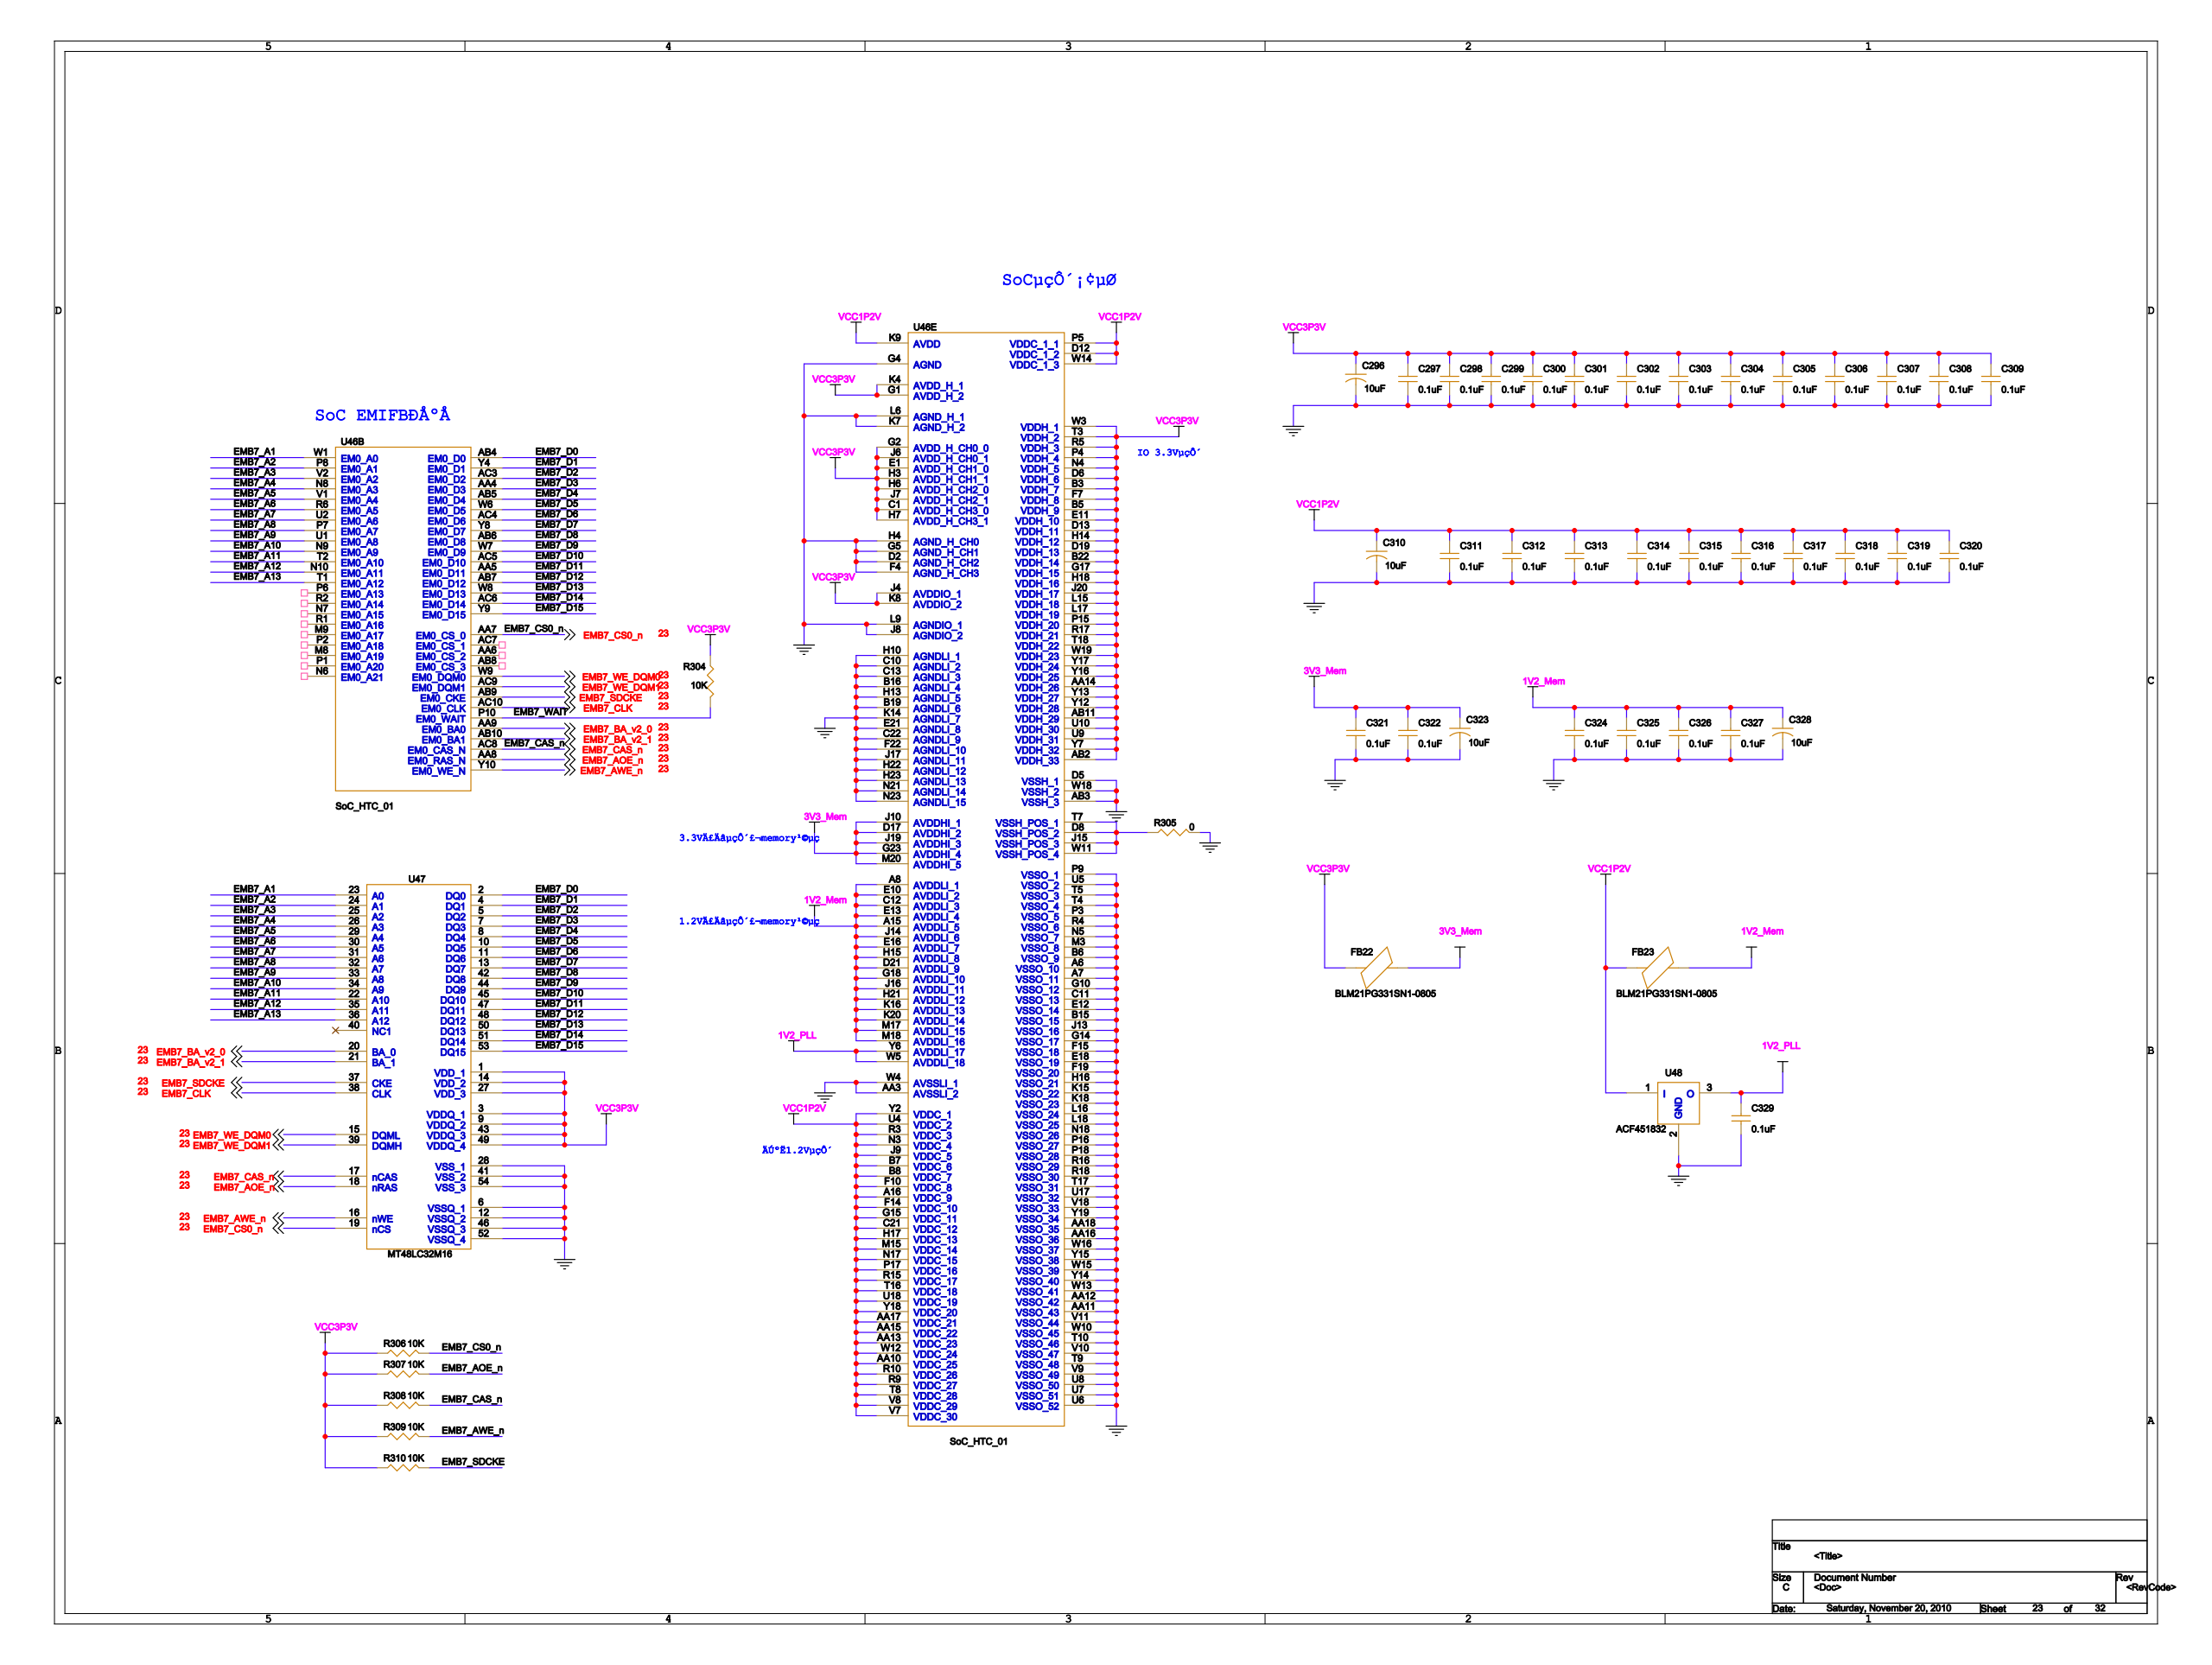Circuit board | Cadence Allegro | 1001 parts | 1318 nets | one sheet of the schematic
Parts on this sheet (reference | value | footprint):
C1 | 10uF | C3216
C10 | 0.1uF | C0402
C21 | 0.1uF | C0402
C22 | 0.1uF | C0402
C296 | 10uF | C3216
C297 | 0.1uF | C0402
C298 | 0.1uF | C0402
C299 | 0.1uF | C0402
C300 | 0.1uF | C0402
C301 | 0.1uF | C0402
C302 | 0.1uF | C0402
C303 | 0.1uF | C0402
C304 | 0.1uF | C0402
C305 | 0.1uF | C0402
C306 | 0.1uF | C0402
C307 | 0.1uF | C0402
C308 | 0.1uF | C0402
C309 | 0.1uF | C0402
C310 | 10uF | C3216
C311 | 0.1uF | C0402
C312 | 0.1uF | C0402
C313 | 0.1uF | C0402
C314 | 0.1uF | C0402
C315 | 0.1uF | C0402
C316 | 0.1uF | C0402
C317 | 0.1uF | C0402
C318 | 0.1uF | C0402
C319 | 0.1uF | C0402
C320 | 0.1uF | C0402
C321 | 0.1uF | C0402
C322 | 0.1uF | C0402
C323 | 10uF | C3216
C324 | 0.1uF | C0402
C325 | 0.1uF | C0402
C326 | 0.1uF | C0402
C327 | 0.1uF | C0402
C328 | 10uF | C3216
C329 | 0.1uF | 0603
FB22 | BLM21PG331SN1-0805 | 1210
FB23 | BLM21PG331SN1-0805 | 1210
R304 | 10K | 0603
R305 | 0 | 0603
R306 | 10K | 0603
R307 | 10K | 0603
R308 | 10K | 0603
R309 | 10K | 0603
R310 | 10K | 0603
U1 | SoC_HTC_01 | L529_XIN
U2 | MT48LC32M16 | TSOP54
U4 | MAX3243 | TSSOP-28
U6 | MT48LC16M16 | TSOP54
U7 | MT48LC16M16 | TSOP54
U8 | DP83848C | DP83848C_48LQFP
U10 | SoC_HTC_01 | L529_XIN
U17 | MT48LC32M16 | TSOP54
U46 | SoC_HTC_01 | L529_XIN
U47 | MT48LC32M16 | TSOP54
U48 | ACF451832 | EMI_FILTER
Nets of these parts (net: part-pin ...):
GND: C1-2 C10-2 C21-2 C22-2 C296-2 C297-2 C298-2 C299-2 C300-2 C301-2 C302-2 C303-2 C304-2 C305-2 C306-2 C307-2 C308-2 C309-2 C310-2 C311-2 C312-2 C313-2 C314-2 C315-2 C316-2 C317-2 C318-2 C319-2 C320-2 C321-2 C322-2 C323-2 C324-2 C325-2 C326-2 C327-2 C328-2 C329-2 R305-2 U48-2 U1-A6 U1-A7 U1-AA3 U1-AA11 U1-AA12 U1-AA16 U1-AA18 U1-AB3 U1-B6 U1-B15 U1-B16 U1-B19 U1-C10 U1-C11 U1-C13 U1-C22 U1-D2 U1-D5 U1-E12 U1-E18 U1-E21 U1-F4 U1-F15 U1-F19 U1-F22 U1-G4 U1-G5 U1-G10 U1-G14 U1-H4 U1-H10 U1-H13 U1-H16 U1-H22 U1-H23 U1-J8 U1-J13 U1-J17 U1-K7 U1-K14 U1-K15 U1-K18 U1-L6 U1-L9 U1-L16 U1-L18 U1-M3 U1-N5 U1-N18 U1-N21 U1-N23 U1-P3 U1-P9 U1-P16 U1-P18 U1-R4 U1-R16 U1-R18 U1-T4 U1-T5 U1-T9 U1-T10 U1-T17 U1-U5 U1-U6 U1-U7 U1-U8 U1-U17 U1-V9 U1-V10 U1-V11 U1-V18 U1-W4 U1-W10 U1-W13 U1-W15 U1-W16 U1-W18 U1-Y14 U1-Y15 U1-Y19 U2-6 U2-12 U2-28 U2-41 U2-46 U2-52 U2-54 U4-23 U4-25 U6-6 U6-12 U6-28 U6-41 U6-46 U6-52 U6-54 U7-6 U7-12 U7-28 U7-41 U7-46 U7-52 U7-54 U8-15 U8-19 U8-35 U8-36 U8-47 U10-A6 U10-A7 U10-AA3 U10-AA11 U10-AA12 U10-AA16 U10-AA18 U10-AB3 U10-B6 U10-B15 U10-B16 U10-B19 U10-C10 U10-C11 U10-C13 U10-C22 U10-D2 U10-D5 U10-E12 U10-E18 U10-E21 U10-F4 U10-F15 U10-F19 U10-F22 U10-G4 U10-G5 U10-G10 U10-G14 U10-H4 U10-H10 U10-H13 U10-H16 U10-H22 U10-H23 U10-J8 U10-J13 U10-J17 U10-K7 U10-K14 U10-K15 U10-K18 U10-L6 U10-L9 U10-L16 U10-L18 U10-M3 U10-N5 U10-N18 U10-N21 U10-N23 U10-P3 U10-P9 U10-P16 U10-P18 U10-R4 U10-R16 U10-R18 U10-T4 U10-T5 U10-T9 U10-T10 U10-T17 U10-U5 U10-U6 U10-U7 U10-U8 U10-U17 U10-V9 U10-V10 U10-V11 U10-V18 U10-W4 U10-W10 U10-W13 U10-W15 U10-W16 U10-W18 U10-Y14 U10-Y15 U10-Y19 U17-6 U17-12 U17-28 U17-41 U17-46 U17-52 U17-54 U46-A6 U46-A7 U46-AA3 U46-AA11 U46-AA12 U46-AA16 U46-AA18 U46-AB3 U46-B6 U46-B15 U46-B16 U46-B19 U46-C10 U46-C11 U46-C13 U46-C22 U46-D2 U46-D5 U46-E12 U46-E18 U46-E21 U46-F4 U46-F15 U46-F19 U46-F22 U46-G4 U46-G5 U46-G10 U46-G14 U46-H4 U46-H10 U46-H13 U46-H16 U46-H22 U46-H23 U46-J8 U46-J13 U46-J17 U46-K7 U46-K14 U46-K15 U46-K18 U46-L6 U46-L9 U46-L16 U46-L18 U46-M3 U46-N5 U46-N18 U46-N21 U46-N23 U46-P3 U46-P9 U46-P16 U46-P18 U46-R4 U46-R16 U46-R18 U46-T4 U46-T5 U46-T9 U46-T10 U46-T17 U46-U5 U46-U6 U46-U7 U46-U8 U46-U17 U46-V9 U46-V10 U46-V11 U46-V18 U46-W4 U46-W10 U46-W13 U46-W15 U46-W16 U46-W18 U46-Y14 U46-Y15 U46-Y19 U47-6 U47-12 U47-28 U47-41 U47-46 U47-52 U47-54
VCC3P3V: C1-1 C10-1 C296-1 C297-1 C298-1 C299-1 C300-1 C301-1 C302-1 C303-1 C304-1 C305-1 C306-1 C307-1 C308-1 C309-1 FB22-1 R304-2 R306-1 R307-1 R308-1 R309-1 R310-1 U1-AA14 U1-AB2 U1-AB11 U1-B3 U1-B5 U1-B22 U1-C1 U1-D6 U1-D13 U1-D19 U1-E1 U1-E11 U1-F7 U1-G1 U1-G2 U1-G17 U1-H3 U1-H6 U1-H7 U1-H14 U1-H18 U1-J4 U1-J6 U1-J7 U1-J20 U1-K4 U1-K8 U1-L15 U1-L17 U1-N4 U1-P4 U1-P15 U1-R5 U1-R17 U1-T3 U1-T18 U1-U9 U1-U10 U1-W3 U1-W19 U1-Y7 U1-Y12 U1-Y13 U1-Y16 U1-Y17 U2-1 U2-3 U2-9 U2-14 U2-27 U2-43 U2-49 U4-22 U4-26 U6-1 U6-3 U6-9 U6-14 U6-27 U6-43 U6-49 U7-1 U7-3 U7-9 U7-14 U7-27 U7-43 U7-49 U8-22 U8-32 U8-48 U10-AA14 U10-AB2 U10-AB11 U10-B3 U10-B5 U10-B22 U10-C1 U10-D6 U10-D13 U10-D19 U10-E1 U10-E11 U10-F7 U10-G1 U10-G2 U10-G17 U10-H3 U10-H6 U10-H7 U10-H14 U10-H18 U10-J4 U10-J6 U10-J7 U10-J20 U10-K4 U10-K8 U10-L15 U10-L17 U10-N4 U10-P4 U10-P15 U10-R5 U10-R17 U10-T3 U10-T18 U10-U9 U10-U10 U10-W3 U10-W19 U10-Y7 U10-Y12 U10-Y13 U10-Y16 U10-Y17 U17-1 U17-3 U17-9 U17-14 U17-27 U17-43 U17-49 U46-AA14 U46-AB2 U46-AB11 U46-B3 U46-B5 U46-B22 U46-C1 U46-D6 U46-D13 U46-D19 U46-E1 U46-E11 U46-F7 U46-G1 U46-G2 U46-G17 U46-H3 U46-H6 U46-H7 U46-H14 U46-H18 U46-J4 U46-J6 U46-J7 U46-J20 U46-K4 U46-K8 U46-L15 U46-L17 U46-N4 U46-P4 U46-P15 U46-R5 U46-R17 U46-T3 U46-T18 U46-U9 U46-U10 U46-W3 U46-W19 U46-Y7 U46-Y12 U46-Y13 U46-Y16 U46-Y17 U47-1 U47-3 U47-9 U47-14 U47-27 U47-43 U47-49
VCC1P2V: C21-1 C22-1 C310-1 C311-1 C312-1 C313-1 C314-1 C315-1 C316-1 C317-1 C318-1 C319-1 C320-1 FB23-1 U48-1 U1-A16 U1-AA10 U1-AA13 U1-AA15 U1-AA17 U1-B7 U1-B8 U1-C21 U1-D12 U1-F10 U1-F14 U1-G15 U1-H17 U1-J9 U1-K9 U1-M15 U1-N3 U1-N17 U1-P5 U1-P17 U1-R3 U1-R9 U1-R10 U1-R15 U1-T8 U1-T16 U1-U4 U1-U18 U1-V7 U1-V8 U1-W12 U1-W14 U1-Y2 U1-Y18 U10-A16 U10-AA10 U10-AA13 U10-AA15 U10-AA17 U10-B7 U10-B8 U10-C21 U10-D12 U10-F10 U10-F14 U10-G15 U10-H17 U10-J9 U10-K9 U10-M15 U10-N3 U10-N17 U10-P5 U10-P17 U10-R3 U10-R9 U10-R10 U10-R15 U10-T8 U10-T16 U10-U4 U10-U18 U10-V7 U10-V8 U10-W12 U10-W14 U10-Y2 U10-Y18 U46-A16 U46-AA10 U46-AA13 U46-AA15 U46-AA17 U46-B7 U46-B8 U46-C21 U46-D12 U46-F10 U46-F14 U46-G15 U46-H17 U46-J9 U46-K9 U46-M15 U46-N3 U46-N17 U46-P5 U46-P17 U46-R3 U46-R9 U46-R10 U46-R15 U46-T8 U46-T16 U46-U4 U46-U18 U46-V7 U46-V8 U46-W12 U46-W14 U46-Y2 U46-Y18
3V3_MEM: C321-1 C322-1 C323-1 FB22-2 U1-D17 U1-G23 U1-J10 U1-J19 U1-M20 U10-D17 U10-G23 U10-J10 U10-J19 U10-M20 U46-D17 U46-G23 U46-J10 U46-J19 U46-M20
1V2_MEM: C324-1 C325-1 C326-1 C327-1 C328-1 FB23-2 U1-A8 U1-A15 U1-C12 U1-D21 U1-E10 U1-E13 U1-E16 U1-G18 U1-H15 U1-H21 U1-J14 U1-J16 U1-K16 U1-K20 U1-M17 U1-M18 U10-A8 U10-A15 U10-C12 U10-D21 U10-E10 U10-E13 U10-E16 U10-G18 U10-H15 U10-H21 U10-J14 U10-J16 U10-K16 U10-K20 U10-M17 U10-M18 U46-A8 U46-A15 U46-C12 U46-D21 U46-E10 U46-E13 U46-E16 U46-G18 U46-H15 U46-H21 U46-J14 U46-J16 U46-K16 U46-K20 U46-M17 U46-M18
1V2_PLL: C329-1 U48-3 U1-W5 U1-Y6 U10-W5 U10-Y6 U46-W5 U46-Y6
EMB7_A1: U46-W1 U47-23
EMB7_A2: U46-P8 U47-24
EMB7_A11: U46-T2 U47-22
EMB7_A12: U46-N10 U47-35
EMB7_A13: U46-T1 U47-36
EMB7_A3: U46-V2 U47-25
EMB7_A4: U46-N8 U47-26
EMB7_A5: U46-V1 U47-29
EMB7_A6: U46-R6 U47-30
EMB7_A7: U46-U2 U47-31
EMB7_A8: U46-P7 U47-32
EMB7_A9: U46-U1 U47-33
EMB7_A10: U46-N9 U47-34
EMB7_CAS_N: R308-2 U46-AC8 U47-17
EMB7_SDCKE: R310-2 U46-AB9 U47-37
EMB7_CLK: U46-AC10 U47-38
EMB7_CS0_N: R306-2 U46-AA7 U47-19
EMB7_D0: U46-AB4 U47-2
EMB7_D1: U46-Y4 U47-4
EMB7_D10: U46-AC5 U47-45
EMB7_D11: U46-AA5 U47-47
EMB7_D12: U46-AB7 U47-48
EMB7_D13: U46-W8 U47-50
EMB7_D14: U46-AC6 U47-51
EMB7_D15: U46-Y9 U47-53
EMB7_D2: U46-AC3 U47-5
EMB7_D3: U46-AA4 U47-7
EMB7_D4: U46-AB5 U47-8
EMB7_D5: U46-W6 U47-10
EMB7_D6: U46-AC4 U47-11
EMB7_D7: U46-Y8 U47-13
EMB7_D8: U46-AB6 U47-42
EMB7_D9: U46-W7 U47-44
EMB7_WE_DQM0: U46-W9 U47-15
EMB7_WE_DQM1: U46-AC9 U47-39
EMB7_AOE_N: R307-2 U46-AA8 U47-18
EMB7_WAIT: R304-1 U46-P10
EMB7_AWE_N: R309-2 U46-Y10 U47-16
N17418822: R305-1 U46-D8 U46-J15 U46-T7 U46-W11